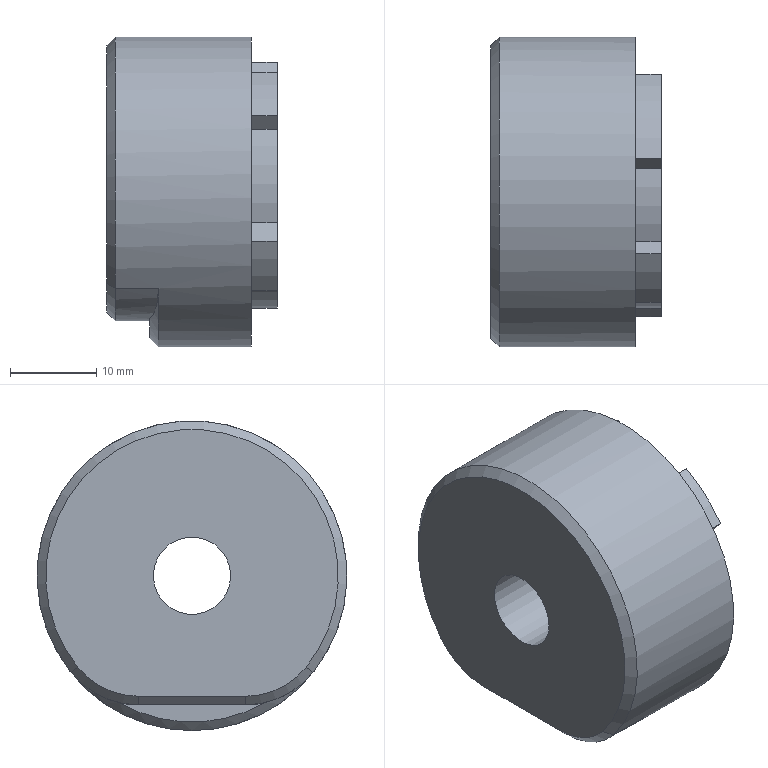Part | STEP file | solid 8 | 1 solid | 32 faces | box 19.849 x 36 x 36 mm | volume 16739 mm3 | plane 15 | cylinder 13 | cone 4 | commonest cylinder face diameters 27.135 x4 31.155 x4 20 x2 9 x1 14 x1 36 x1